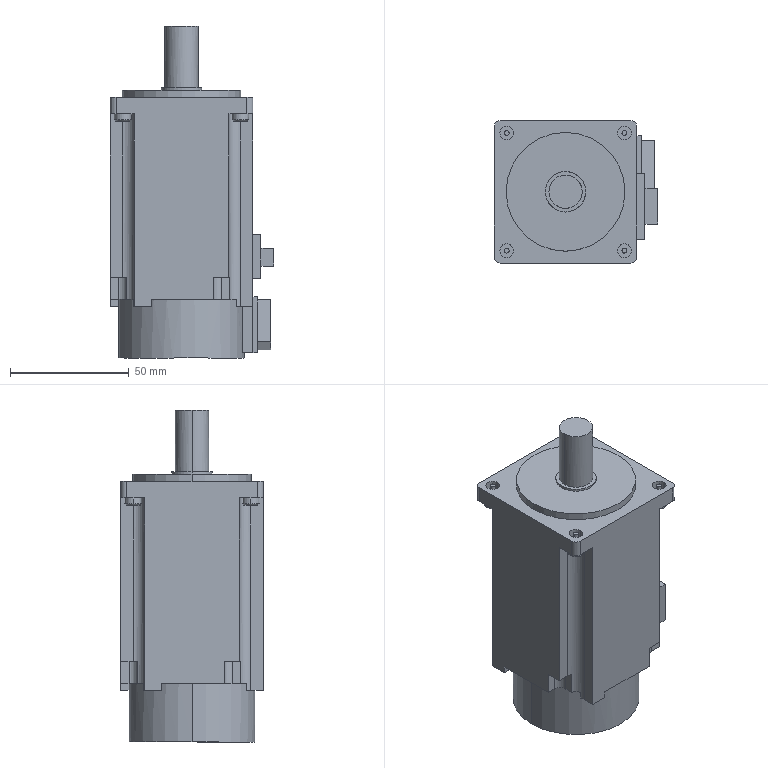Part | SolidWorks | features BaseBody 1 | 1 solid | 168 faces | box 68.8 x 60 x 139.7 mm | volume 348591 mm3 | plane 112 | cylinder 48 | cone 8 | commonest cylinder face diameters 7 x16 2 x8 5.8 x8 5 x4 9.6 x4 14 x2